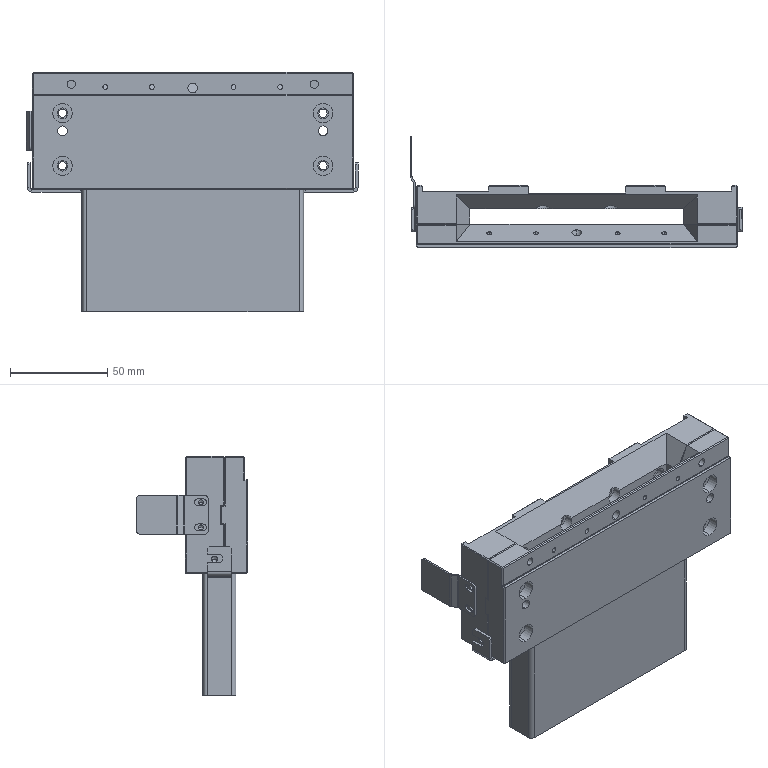Part | SolidWorks | 4 solids | 400 faces | box 170.787 x 57.213 x 123 mm | volume 228547 mm3 | plane 235 | cylinder 146 | cone 19 | commonest cylinder face diameters 4.5 x26 8 x24 2.5 x16 4.2 x12 5 x12 1.473 x10